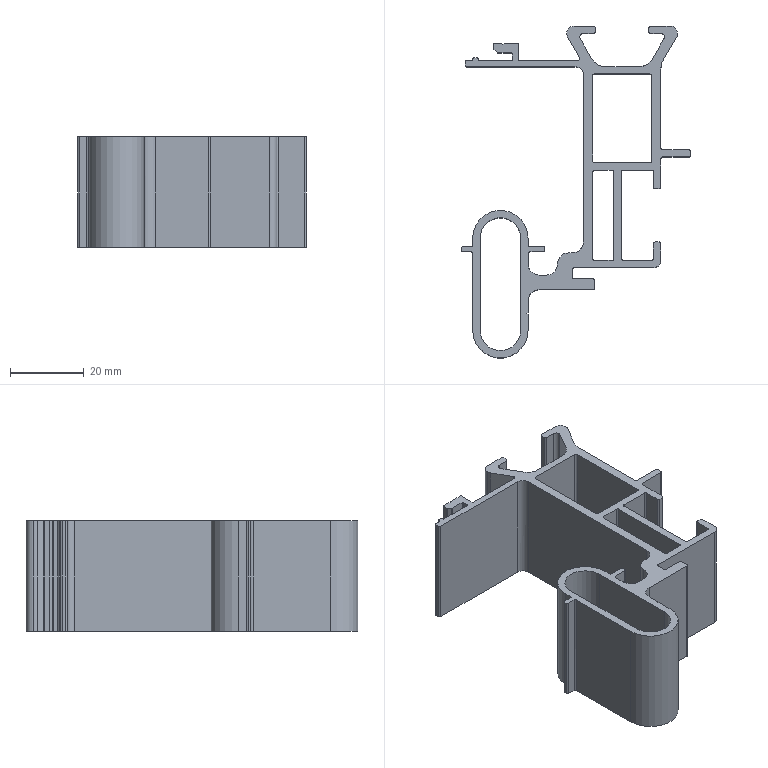Part | STEP file | 51E-01179JG10 | 1 solid | 150 faces | box 62 x 90 x 30 mm | volume 25669 mm3 | plane 79 | cylinder 71 | commonest cylinder face diameters 1 x40 0.4 x7 4 x6 6 x5 2 x4 8 x2